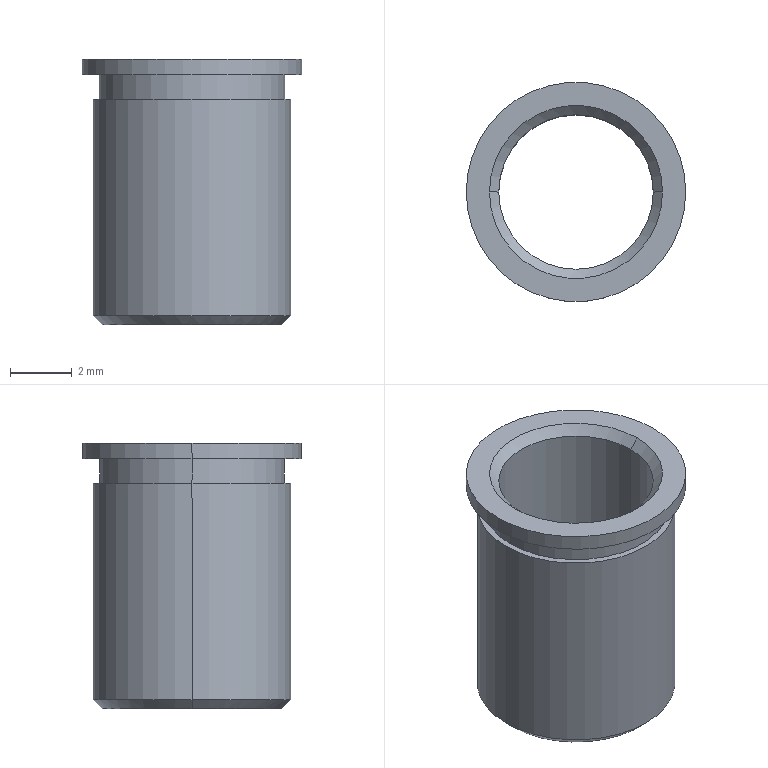Part | STEP file | 1 solid | 18 faces | box 7.1 x 7.1 x 8.6 mm | volume 106.048 mm3 | cylinder 8 | cone 6 | plane 4 | commonest cylinder face diameters 5 x2 6 x2 6.4 x2 7.1 x2
STEP:
#1=CARTESIAN_POINT('',(-2.9,0.,-8.6));
#2=VERTEX_POINT('',#1);
#3=CARTESIAN_POINT('',(-3.2,0.,-8.3));
#4=VERTEX_POINT('',#3);
#5=CARTESIAN_POINT('',(-2.9,0.,-8.6));
#6=DIRECTION('',(-0.7071,0.,0.7071));
#7=VECTOR('',#6,1000.);
#8=LINE('',#5,#7);
#9=EDGE_CURVE('',#2,#4,#8,.T.);
#10=ORIENTED_EDGE('',*,*,#9,.F.);
#11=CARTESIAN_POINT('',(2.9,0.,-8.6));
#12=VERTEX_POINT('',#11);
#13=CARTESIAN_POINT('',(0.,0.,-8.6));
#14=DIRECTION('',(0.,0.,-1.));
#15=DIRECTION('',(-1.,0.,0.));
#16=AXIS2_PLACEMENT_3D('',#13,#14,#15);
#17=CIRCLE('',#16,2.9);
#18=EDGE_CURVE('',#12,#2,#17,.T.);
#19=ORIENTED_EDGE('',*,*,#18,.F.);
#20=CARTESIAN_POINT('',(3.2,0.,-8.3));
#21=VERTEX_POINT('',#20);
#22=CARTESIAN_POINT('',(2.9,0.,-8.6));
#23=DIRECTION('',(0.7071,0.,0.7071));
#24=VECTOR('',#23,1000.);
#25=LINE('',#22,#24);
#26=EDGE_CURVE('',#12,#21,#25,.T.);
#27=ORIENTED_EDGE('',*,*,#26,.T.);
#28=CARTESIAN_POINT('',(0.,0.,-8.3));
#29=DIRECTION('',(0.,0.,1.));
#30=DIRECTION('',(-1.,0.,0.));
#31=AXIS2_PLACEMENT_3D('',#28,#29,#30);
#32=CIRCLE('',#31,3.2);
#33=EDGE_CURVE('',#4,#21,#32,.T.);
#34=ORIENTED_EDGE('',*,*,#33,.F.);
#35=EDGE_LOOP('',(#10,#19,#27,#34));
#36=FACE_OUTER_BOUND('',#35,.T.);
#37=CARTESIAN_POINT('',(0.,0.,-8.6));
#38=DIRECTION('',(0.,0.,1.));
#39=DIRECTION('',(1.,0.,0.));
#40=AXIS2_PLACEMENT_3D('',#37,#38,#39);
#41=CONICAL_SURFACE('',#40,2.9,0.7854);
#42=ADVANCED_FACE('',(#36),#41,.T.);
#43=CARTESIAN_POINT('',(-2.5,0.,-0.3));
#44=VERTEX_POINT('',#43);
#45=CARTESIAN_POINT('',(-2.8,0.,0.));
#46=VERTEX_POINT('',#45);
#47=CARTESIAN_POINT('',(-2.8,0.,0.));
#48=DIRECTION('',(-0.7071,0.,0.7071));
#49=VECTOR('',#48,1000.);
#50=LINE('',#47,#49);
#51=EDGE_CURVE('',#44,#46,#50,.T.);
#52=ORIENTED_EDGE('',*,*,#51,.F.);
#53=CARTESIAN_POINT('',(2.5,0.,-0.3));
#54=VERTEX_POINT('',#53);
#55=CARTESIAN_POINT('',(0.,0.,-0.3));
#56=DIRECTION('',(0.,0.,1.));
#57=DIRECTION('',(1.,0.,0.));
#58=AXIS2_PLACEMENT_3D('',#55,#56,#57);
#59=CIRCLE('',#58,2.5);
#60=EDGE_CURVE('',#54,#44,#59,.T.);
#61=ORIENTED_EDGE('',*,*,#60,.F.);
#62=CARTESIAN_POINT('',(2.8,0.,0.));
#63=VERTEX_POINT('',#62);
#64=CARTESIAN_POINT('',(2.8,0.,0.));
#65=DIRECTION('',(0.7071,0.,0.7071));
#66=VECTOR('',#65,1000.);
#67=LINE('',#64,#66);
#68=EDGE_CURVE('',#54,#63,#67,.T.);
#69=ORIENTED_EDGE('',*,*,#68,.T.);
#70=CARTESIAN_POINT('',(0.,0.,0.));
#71=DIRECTION('',(0.,0.,-1.));
#72=DIRECTION('',(1.,0.,0.));
#73=AXIS2_PLACEMENT_3D('',#70,#71,#72);
#74=CIRCLE('',#73,2.8);
#75=EDGE_CURVE('',#46,#63,#74,.T.);
#76=ORIENTED_EDGE('',*,*,#75,.F.);
#77=EDGE_LOOP('',(#52,#61,#69,#76));
#78=FACE_OUTER_BOUND('',#77,.T.);
#79=CARTESIAN_POINT('',(0.,0.,0.));
#80=DIRECTION('',(0.,0.,1.));
#81=DIRECTION('',(1.,0.,0.));
#82=AXIS2_PLACEMENT_3D('',#79,#80,#81);
#83=CONICAL_SURFACE('',#82,2.8,0.7854);
#84=ADVANCED_FACE('',(#78),#83,.F.);
#85=CARTESIAN_POINT('',(2.5,0.,-8.3));
#86=VERTEX_POINT('',#85);
#87=CARTESIAN_POINT('',(2.8,0.,-8.6));
#88=VERTEX_POINT('',#87);
#89=CARTESIAN_POINT('',(2.5,0.,-8.3));
#90=DIRECTION('',(0.7071,0.,-0.7071));
#91=VECTOR('',#90,1000.);
#92=LINE('',#89,#91);
#93=EDGE_CURVE('',#86,#88,#92,.T.);
#94=ORIENTED_EDGE('',*,*,#93,.F.);
#95=CARTESIAN_POINT('',(-2.5,0.,-8.3));
#96=VERTEX_POINT('',#95);
#97=CARTESIAN_POINT('',(0.,0.,-8.3));
#98=DIRECTION('',(0.,0.,-1.));
#99=DIRECTION('',(-1.,0.,0.));
#100=AXIS2_PLACEMENT_3D('',#97,#98,#99);
#101=CIRCLE('',#100,2.5);
#102=EDGE_CURVE('',#96,#86,#101,.T.);
#103=ORIENTED_EDGE('',*,*,#102,.F.);
#104=CARTESIAN_POINT('',(-2.8,0.,-8.6));
#105=VERTEX_POINT('',#104);
#106=CARTESIAN_POINT('',(-2.5,0.,-8.3));
#107=DIRECTION('',(-0.7071,0.,-0.7071));
#108=VECTOR('',#107,1000.);
#109=LINE('',#106,#108);
#110=EDGE_CURVE('',#96,#105,#109,.T.);
#111=ORIENTED_EDGE('',*,*,#110,.T.);
#112=CARTESIAN_POINT('',(0.,0.,-8.6));
#113=DIRECTION('',(0.,0.,1.));
#114=DIRECTION('',(-1.,0.,0.));
#115=AXIS2_PLACEMENT_3D('',#112,#113,#114);
#116=CIRCLE('',#115,2.8);
#117=EDGE_CURVE('',#88,#105,#116,.T.);
#118=ORIENTED_EDGE('',*,*,#117,.F.);
#119=EDGE_LOOP('',(#94,#103,#111,#118));
#120=FACE_OUTER_BOUND('',#119,.T.);
#121=CARTESIAN_POINT('',(0.,0.,-8.3));
#122=DIRECTION('',(0.,0.,-1.));
#123=DIRECTION('',(-1.,0.,0.));
#124=AXIS2_PLACEMENT_3D('',#121,#122,#123);
#125=CONICAL_SURFACE('',#124,2.5,0.7854);
#126=ADVANCED_FACE('',(#120),#125,.F.);
#127=CARTESIAN_POINT('',(2.5,0.,0.));
#128=DIRECTION('',(0.,0.,-1.));
#129=VECTOR('',#128,1000.);
#130=LINE('',#127,#129);
#131=EDGE_CURVE('',#54,#86,#130,.T.);
#132=ORIENTED_EDGE('',*,*,#131,.F.);
#133=ORIENTED_EDGE('',*,*,#60,.T.);
#134=CARTESIAN_POINT('',(-2.5,0.,0.));
#135=DIRECTION('',(0.,0.,-1.));
#136=VECTOR('',#135,1000.);
#137=LINE('',#134,#136);
#138=EDGE_CURVE('',#44,#96,#137,.T.);
#139=ORIENTED_EDGE('',*,*,#138,.T.);
#140=ORIENTED_EDGE('',*,*,#102,.T.);
#141=EDGE_LOOP('',(#132,#133,#139,#140));
#142=FACE_OUTER_BOUND('',#141,.T.);
#143=CARTESIAN_POINT('',(0.,0.,0.));
#144=DIRECTION('',(0.,0.,-1.));
#145=DIRECTION('',(-1.,0.,0.));
#146=AXIS2_PLACEMENT_3D('',#143,#144,#145);
#147=CYLINDRICAL_SURFACE('',#146,2.5);
#148=ADVANCED_FACE('',(#142),#147,.F.);
#149=CARTESIAN_POINT('',(0.,0.,0.));
#150=DIRECTION('',(0.,0.,-1.));
#151=DIRECTION('',(1.,0.,0.));
#152=AXIS2_PLACEMENT_3D('',#149,#150,#151);
#153=CIRCLE('',#152,2.8);
#154=EDGE_CURVE('',#63,#46,#153,.T.);
#155=ORIENTED_EDGE('',*,*,#154,.T.);
#156=ORIENTED_EDGE('',*,*,#75,.T.);
#157=EDGE_LOOP('',(#155,#156));
#158=FACE_BOUND('',#157,.T.);
#159=CARTESIAN_POINT('',(-3.55,0.,0.));
#160=VERTEX_POINT('',#159);
#161=CARTESIAN_POINT('',(3.55,0.,0.));
#162=VERTEX_POINT('',#161);
#163=CARTESIAN_POINT('',(0.,0.,0.));
#164=DIRECTION('',(0.,0.,-1.));
#165=DIRECTION('',(-1.,0.,0.));
#166=AXIS2_PLACEMENT_3D('',#163,#164,#165);
#167=CIRCLE('',#166,3.55);
#168=EDGE_CURVE('',#160,#162,#167,.T.);
#169=ORIENTED_EDGE('',*,*,#168,.F.);
#170=CARTESIAN_POINT('',(0.,0.,0.));
#171=DIRECTION('',(0.,0.,-1.));
#172=DIRECTION('',(-1.,0.,0.));
#173=AXIS2_PLACEMENT_3D('',#170,#171,#172);
#174=CIRCLE('',#173,3.55);
#175=EDGE_CURVE('',#162,#160,#174,.T.);
#176=ORIENTED_EDGE('',*,*,#175,.F.);
#177=EDGE_LOOP('',(#169,#176));
#178=FACE_OUTER_BOUND('',#177,.T.);
#179=CARTESIAN_POINT('',(-3.55,0.,0.));
#180=DIRECTION('',(0.,0.,1.));
#181=DIRECTION('',(1.,0.,0.));
#182=AXIS2_PLACEMENT_3D('',#179,#180,#181);
#183=PLANE('',#182);
#184=ADVANCED_FACE('',(#158,#178),#183,.T.);
#185=CARTESIAN_POINT('',(3.55,0.,-0.5));
#186=VERTEX_POINT('',#185);
#187=CARTESIAN_POINT('',(3.55,0.,-11.396));
#188=DIRECTION('',(0.,0.,-1.));
#189=VECTOR('',#188,1000.);
#190=LINE('',#187,#189);
#191=EDGE_CURVE('',#162,#186,#190,.T.);
#192=ORIENTED_EDGE('',*,*,#191,.F.);
#193=ORIENTED_EDGE('',*,*,#175,.T.);
#194=CARTESIAN_POINT('',(-3.55,0.,-0.5));
#195=VERTEX_POINT('',#194);
#196=CARTESIAN_POINT('',(-3.55,0.,-11.396));
#197=DIRECTION('',(0.,0.,-1.));
#198=VECTOR('',#197,1000.);
#199=LINE('',#196,#198);
#200=EDGE_CURVE('',#160,#195,#199,.T.);
#201=ORIENTED_EDGE('',*,*,#200,.T.);
#202=CARTESIAN_POINT('',(0.,0.,-0.5));
#203=DIRECTION('',(0.,0.,-1.));
#204=DIRECTION('',(-1.,0.,0.));
#205=AXIS2_PLACEMENT_3D('',#202,#203,#204);
#206=CIRCLE('',#205,3.55);
#207=EDGE_CURVE('',#186,#195,#206,.T.);
#208=ORIENTED_EDGE('',*,*,#207,.F.);
#209=EDGE_LOOP('',(#192,#193,#201,#208));
#210=FACE_OUTER_BOUND('',#209,.T.);
#211=CARTESIAN_POINT('',(0.,0.,-11.396));
#212=DIRECTION('',(0.,0.,-1.));
#213=DIRECTION('',(-1.,0.,0.));
#214=AXIS2_PLACEMENT_3D('',#211,#212,#213);
#215=CYLINDRICAL_SURFACE('',#214,3.55);
#216=ADVANCED_FACE('',(#210),#215,.T.);
#217=CARTESIAN_POINT('',(-3.,0.,-0.5));
#218=VERTEX_POINT('',#217);
#219=CARTESIAN_POINT('',(3.,0.,-0.5));
#220=VERTEX_POINT('',#219);
#221=CARTESIAN_POINT('',(0.,0.,-0.5));
#222=DIRECTION('',(0.,0.,-1.));
#223=DIRECTION('',(-1.,0.,0.));
#224=AXIS2_PLACEMENT_3D('',#221,#222,#223);
#225=CIRCLE('',#224,3.);
#226=EDGE_CURVE('',#218,#220,#225,.T.);
#227=ORIENTED_EDGE('',*,*,#226,.F.);
#228=CARTESIAN_POINT('',(0.,0.,-0.5));
#229=DIRECTION('',(0.,0.,-1.));
#230=DIRECTION('',(-1.,0.,0.));
#231=AXIS2_PLACEMENT_3D('',#228,#229,#230);
#232=CIRCLE('',#231,3.);
#233=EDGE_CURVE('',#220,#218,#232,.T.);
#234=ORIENTED_EDGE('',*,*,#233,.F.);
#235=EDGE_LOOP('',(#227,#234));
#236=FACE_BOUND('',#235,.T.);
#237=CARTESIAN_POINT('',(0.,0.,-0.5));
#238=DIRECTION('',(0.,0.,-1.));
#239=DIRECTION('',(-1.,0.,0.));
#240=AXIS2_PLACEMENT_3D('',#237,#238,#239);
#241=CIRCLE('',#240,3.55);
#242=EDGE_CURVE('',#195,#186,#241,.T.);
#243=ORIENTED_EDGE('',*,*,#242,.T.);
#244=ORIENTED_EDGE('',*,*,#207,.T.);
#245=EDGE_LOOP('',(#243,#244));
#246=FACE_OUTER_BOUND('',#245,.T.);
#247=CARTESIAN_POINT('',(-3.,0.,-0.5));
#248=DIRECTION('',(0.,0.,-1.));
#249=DIRECTION('',(0.,-1.,0.));
#250=AXIS2_PLACEMENT_3D('',#247,#248,#249);
#251=PLANE('',#250);
#252=ADVANCED_FACE('',(#236,#246),#251,.T.);
#253=CARTESIAN_POINT('',(3.,0.,-1.3));
#254=VERTEX_POINT('',#253);
#255=CARTESIAN_POINT('',(3.,0.,-11.396));
#256=DIRECTION('',(0.,0.,-1.));
#257=VECTOR('',#256,1000.);
#258=LINE('',#255,#257);
#259=EDGE_CURVE('',#220,#254,#258,.T.);
#260=ORIENTED_EDGE('',*,*,#259,.F.);
#261=ORIENTED_EDGE('',*,*,#233,.T.);
#262=CARTESIAN_POINT('',(-3.,0.,-1.3));
#263=VERTEX_POINT('',#262);
#264=CARTESIAN_POINT('',(-3.,0.,-11.396));
#265=DIRECTION('',(0.,0.,-1.));
#266=VECTOR('',#265,1000.);
#267=LINE('',#264,#266);
#268=EDGE_CURVE('',#218,#263,#267,.T.);
#269=ORIENTED_EDGE('',*,*,#268,.T.);
#270=CARTESIAN_POINT('',(0.,0.,-1.3));
#271=DIRECTION('',(0.,0.,-1.));
#272=DIRECTION('',(-1.,0.,0.));
#273=AXIS2_PLACEMENT_3D('',#270,#271,#272);
#274=CIRCLE('',#273,3.);
#275=EDGE_CURVE('',#254,#263,#274,.T.);
#276=ORIENTED_EDGE('',*,*,#275,.F.);
#277=EDGE_LOOP('',(#260,#261,#269,#276));
#278=FACE_OUTER_BOUND('',#277,.T.);
#279=CARTESIAN_POINT('',(0.,0.,-11.396));
#280=DIRECTION('',(0.,0.,-1.));
#281=DIRECTION('',(-1.,0.,0.));
#282=AXIS2_PLACEMENT_3D('',#279,#280,#281);
#283=CYLINDRICAL_SURFACE('',#282,3.);
#284=ADVANCED_FACE('',(#278),#283,.T.);
#285=CARTESIAN_POINT('',(0.,0.,-1.3));
#286=DIRECTION('',(0.,0.,-1.));
#287=DIRECTION('',(-1.,0.,0.));
#288=AXIS2_PLACEMENT_3D('',#285,#286,#287);
#289=CIRCLE('',#288,3.);
#290=EDGE_CURVE('',#263,#254,#289,.T.);
#291=ORIENTED_EDGE('',*,*,#290,.T.);
#292=ORIENTED_EDGE('',*,*,#275,.T.);
#293=EDGE_LOOP('',(#291,#292));
#294=FACE_BOUND('',#293,.T.);
#295=CARTESIAN_POINT('',(-3.2,0.,-1.3));
#296=VERTEX_POINT('',#295);
#297=CARTESIAN_POINT('',(3.2,0.,-1.3));
#298=VERTEX_POINT('',#297);
#299=CARTESIAN_POINT('',(0.,0.,-1.3));
#300=DIRECTION('',(0.,0.,-1.));
#301=DIRECTION('',(-1.,0.,0.));
#302=AXIS2_PLACEMENT_3D('',#299,#300,#301);
#303=CIRCLE('',#302,3.2);
#304=EDGE_CURVE('',#296,#298,#303,.T.);
#305=ORIENTED_EDGE('',*,*,#304,.F.);
#306=CARTESIAN_POINT('',(0.,0.,-1.3));
#307=DIRECTION('',(0.,0.,-1.));
#308=DIRECTION('',(-1.,0.,0.));
#309=AXIS2_PLACEMENT_3D('',#306,#307,#308);
#310=CIRCLE('',#309,3.2);
#311=EDGE_CURVE('',#298,#296,#310,.T.);
#312=ORIENTED_EDGE('',*,*,#311,.F.);
#313=EDGE_LOOP('',(#305,#312));
#314=FACE_OUTER_BOUND('',#313,.T.);
#315=CARTESIAN_POINT('',(-3.2,0.,-1.3));
#316=DIRECTION('',(0.,0.,1.));
#317=DIRECTION('',(1.,0.,0.));
#318=AXIS2_PLACEMENT_3D('',#315,#316,#317);
#319=PLANE('',#318);
#320=ADVANCED_FACE('',(#294,#314),#319,.T.);
#321=CARTESIAN_POINT('',(3.2,0.,-11.396));
#322=DIRECTION('',(0.,0.,-1.));
#323=VECTOR('',#322,1000.);
#324=LINE('',#321,#323);
#325=EDGE_CURVE('',#298,#21,#324,.T.);
#326=ORIENTED_EDGE('',*,*,#325,.F.);
#327=ORIENTED_EDGE('',*,*,#311,.T.);
#328=CARTESIAN_POINT('',(-3.2,0.,-11.396));
#329=DIRECTION('',(0.,0.,-1.));
#330=VECTOR('',#329,1000.);
#331=LINE('',#328,#330);
#332=EDGE_CURVE('',#296,#4,#331,.T.);
#333=ORIENTED_EDGE('',*,*,#332,.T.);
#334=ORIENTED_EDGE('',*,*,#33,.T.);
#335=EDGE_LOOP('',(#326,#327,#333,#334));
#336=FACE_OUTER_BOUND('',#335,.T.);
#337=CARTESIAN_POINT('',(0.,0.,-11.396));
#338=DIRECTION('',(0.,0.,-1.));
#339=DIRECTION('',(-1.,0.,0.));
#340=AXIS2_PLACEMENT_3D('',#337,#338,#339);
#341=CYLINDRICAL_SURFACE('',#340,3.2);
#342=ADVANCED_FACE('',(#336),#341,.T.);
#343=CARTESIAN_POINT('',(0.,0.,-8.6));
#344=DIRECTION('',(0.,0.,1.));
#345=DIRECTION('',(-1.,0.,0.));
#346=AXIS2_PLACEMENT_3D('',#343,#344,#345);
#347=CIRCLE('',#346,2.8);
#348=EDGE_CURVE('',#105,#88,#347,.T.);
#349=ORIENTED_EDGE('',*,*,#348,.T.);
#350=ORIENTED_EDGE('',*,*,#117,.T.);
#351=EDGE_LOOP('',(#349,#350));
#352=FACE_BOUND('',#351,.T.);
#353=ORIENTED_EDGE('',*,*,#18,.T.);
#354=CARTESIAN_POINT('',(0.,0.,-8.6));
#355=DIRECTION('',(0.,0.,-1.));
#356=DIRECTION('',(-1.,0.,0.));
#357=AXIS2_PLACEMENT_3D('',#354,#355,#356);
#358=CIRCLE('',#357,2.9);
#359=EDGE_CURVE('',#2,#12,#358,.T.);
#360=ORIENTED_EDGE('',*,*,#359,.T.);
#361=EDGE_LOOP('',(#353,#360));
#362=FACE_OUTER_BOUND('',#361,.T.);
#363=CARTESIAN_POINT('',(0.,0.,-8.6));
#364=DIRECTION('',(0.,0.,-1.));
#365=DIRECTION('',(0.,-1.,0.));
#366=AXIS2_PLACEMENT_3D('',#363,#364,#365);
#367=PLANE('',#366);
#368=ADVANCED_FACE('',(#352,#362),#367,.T.);
#369=ORIENTED_EDGE('',*,*,#304,.T.);
#370=ORIENTED_EDGE('',*,*,#325,.T.);
#371=CARTESIAN_POINT('',(0.,0.,-8.3));
#372=DIRECTION('',(0.,0.,1.));
#373=DIRECTION('',(-1.,0.,0.));
#374=AXIS2_PLACEMENT_3D('',#371,#372,#373);
#375=CIRCLE('',#374,3.2);
#376=EDGE_CURVE('',#21,#4,#375,.T.);
#377=ORIENTED_EDGE('',*,*,#376,.T.);
#378=ORIENTED_EDGE('',*,*,#332,.F.);
#379=EDGE_LOOP('',(#369,#370,#377,#378));
#380=FACE_OUTER_BOUND('',#379,.T.);
#381=CARTESIAN_POINT('',(0.,0.,-11.396));
#382=DIRECTION('',(0.,0.,-1.));
#383=DIRECTION('',(-1.,0.,0.));
#384=AXIS2_PLACEMENT_3D('',#381,#382,#383);
#385=CYLINDRICAL_SURFACE('',#384,3.2);
#386=ADVANCED_FACE('',(#380),#385,.T.);
#387=ORIENTED_EDGE('',*,*,#226,.T.);
#388=ORIENTED_EDGE('',*,*,#259,.T.);
#389=ORIENTED_EDGE('',*,*,#290,.F.);
#390=ORIENTED_EDGE('',*,*,#268,.F.);
#391=EDGE_LOOP('',(#387,#388,#389,#390));
#392=FACE_OUTER_BOUND('',#391,.T.);
#393=CARTESIAN_POINT('',(0.,0.,-11.396));
#394=DIRECTION('',(0.,0.,-1.));
#395=DIRECTION('',(-1.,0.,0.));
#396=AXIS2_PLACEMENT_3D('',#393,#394,#395);
#397=CYLINDRICAL_SURFACE('',#396,3.);
#398=ADVANCED_FACE('',(#392),#397,.T.);
#399=ORIENTED_EDGE('',*,*,#168,.T.);
#400=ORIENTED_EDGE('',*,*,#191,.T.);
#401=ORIENTED_EDGE('',*,*,#242,.F.);
#402=ORIENTED_EDGE('',*,*,#200,.F.);
#403=EDGE_LOOP('',(#399,#400,#401,#402));
#404=FACE_OUTER_BOUND('',#403,.T.);
#405=CARTESIAN_POINT('',(0.,0.,-11.396));
#406=DIRECTION('',(0.,0.,-1.));
#407=DIRECTION('',(-1.,0.,0.));
#408=AXIS2_PLACEMENT_3D('',#405,#406,#407);
#409=CYLINDRICAL_SURFACE('',#408,3.55);
#410=ADVANCED_FACE('',(#404),#409,.T.);
#411=CARTESIAN_POINT('',(0.,0.,-0.3));
#412=DIRECTION('',(0.,0.,1.));
#413=DIRECTION('',(1.,0.,0.));
#414=AXIS2_PLACEMENT_3D('',#411,#412,#413);
#415=CIRCLE('',#414,2.5);
#416=EDGE_CURVE('',#44,#54,#415,.T.);
#417=ORIENTED_EDGE('',*,*,#416,.T.);
#418=ORIENTED_EDGE('',*,*,#131,.T.);
#419=CARTESIAN_POINT('',(0.,0.,-8.3));
#420=DIRECTION('',(0.,0.,-1.));
#421=DIRECTION('',(-1.,0.,0.));
#422=AXIS2_PLACEMENT_3D('',#419,#420,#421);
#423=CIRCLE('',#422,2.5);
#424=EDGE_CURVE('',#86,#96,#423,.T.);
#425=ORIENTED_EDGE('',*,*,#424,.T.);
#426=ORIENTED_EDGE('',*,*,#138,.F.);
#427=EDGE_LOOP('',(#417,#418,#425,#426));
#428=FACE_OUTER_BOUND('',#427,.T.);
#429=CARTESIAN_POINT('',(0.,0.,0.));
#430=DIRECTION('',(0.,0.,-1.));
#431=DIRECTION('',(-1.,0.,0.));
#432=AXIS2_PLACEMENT_3D('',#429,#430,#431);
#433=CYLINDRICAL_SURFACE('',#432,2.5);
#434=ADVANCED_FACE('',(#428),#433,.F.);
#435=ORIENTED_EDGE('',*,*,#424,.F.);
#436=ORIENTED_EDGE('',*,*,#93,.T.);
#437=ORIENTED_EDGE('',*,*,#348,.F.);
#438=ORIENTED_EDGE('',*,*,#110,.F.);
#439=EDGE_LOOP('',(#435,#436,#437,#438));
#440=FACE_OUTER_BOUND('',#439,.T.);
#441=CARTESIAN_POINT('',(0.,0.,-8.3));
#442=DIRECTION('',(0.,0.,-1.));
#443=DIRECTION('',(-1.,0.,0.));
#444=AXIS2_PLACEMENT_3D('',#441,#442,#443);
#445=CONICAL_SURFACE('',#444,2.5,0.7854);
#446=ADVANCED_FACE('',(#440),#445,.F.);
#447=ORIENTED_EDGE('',*,*,#416,.F.);
#448=ORIENTED_EDGE('',*,*,#51,.T.);
#449=ORIENTED_EDGE('',*,*,#154,.F.);
#450=ORIENTED_EDGE('',*,*,#68,.F.);
#451=EDGE_LOOP('',(#447,#448,#449,#450));
#452=FACE_OUTER_BOUND('',#451,.T.);
#453=CARTESIAN_POINT('',(0.,0.,0.));
#454=DIRECTION('',(0.,0.,1.));
#455=DIRECTION('',(1.,0.,0.));
#456=AXIS2_PLACEMENT_3D('',#453,#454,#455);
#457=CONICAL_SURFACE('',#456,2.8,0.7854);
#458=ADVANCED_FACE('',(#452),#457,.F.);
#459=ORIENTED_EDGE('',*,*,#359,.F.);
#460=ORIENTED_EDGE('',*,*,#9,.T.);
#461=ORIENTED_EDGE('',*,*,#376,.F.);
#462=ORIENTED_EDGE('',*,*,#26,.F.);
#463=EDGE_LOOP('',(#459,#460,#461,#462));
#464=FACE_OUTER_BOUND('',#463,.T.);
#465=CARTESIAN_POINT('',(0.,0.,-8.6));
#466=DIRECTION('',(0.,0.,1.));
#467=DIRECTION('',(1.,0.,0.));
#468=AXIS2_PLACEMENT_3D('',#465,#466,#467);
#469=CONICAL_SURFACE('',#468,2.9,0.7854);
#470=ADVANCED_FACE('',(#464),#469,.T.);
#471=CLOSED_SHELL('',(#42,#84,#126,#148,#184,#216,#252,#284,#320,#342,#368,#386,#398,#410,#434,#446,#458,#470));
#472=MANIFOLD_SOLID_BREP('',#471);
#473=CARTESIAN_POINT('',(0.,0.,0.));
#474=DIRECTION('',(0.,0.,1.));
#475=DIRECTION('',(1.,0.,0.));
#476=AXIS2_PLACEMENT_3D('',#473,#474,#475);
#477=(LENGTH_UNIT()NAMED_UNIT(*)SI_UNIT(.MILLI.,.METRE.));
#478=UNCERTAINTY_MEASURE_WITH_UNIT(LENGTH_MEASURE(0.00001),#477,'','');
#479=(NAMED_UNIT(*)PLANE_ANGLE_UNIT()SI_UNIT($,.RADIAN.));
#480=(NAMED_UNIT(*)SI_UNIT($,.STERADIAN.)SOLID_ANGLE_UNIT());
#481=(GEOMETRIC_REPRESENTATION_CONTEXT(3)GLOBAL_UNCERTAINTY_ASSIGNED_CONTEXT((#478))GLOBAL_UNIT_ASSIGNED_CONTEXT((#477,#479,#480))REPRESENTATION_CONTEXT('',''));
#482=ADVANCED_BREP_SHAPE_REPRESENTATION('',(#472,#476),#481);